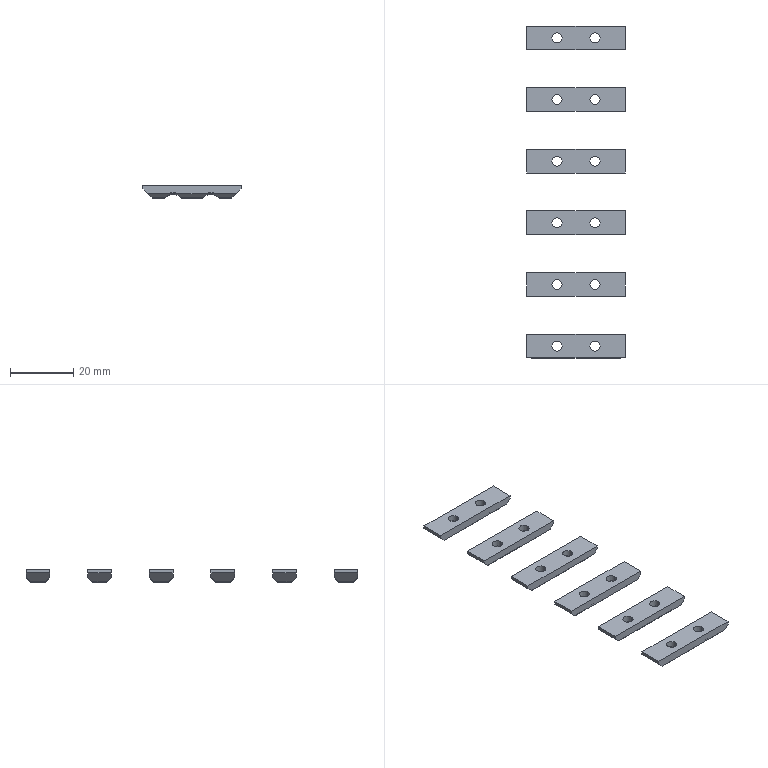NC program | NX | posted with a generic post | part box 31 x 105 x 4 mm
Lines 5449 to 7045 of 12738:
(PLANAR_MILL , TOOL : D0.3)
N10860 T17 M6
N10862 G54
N10864 G17 G0 G90 X-45.35 Y-12.5 S9500 M3
N10866 G43 Z30. H17
N10868 Z0.97
N10870 G94 G1 Z-0.03 F750.
N10872 X-46.5
N10874 X-51.
N10876 X-52.15
N10878 Z0.97
N10880 G0 Z30.
N10882 X-45.35 Y-12.
N10884 Z0.97
N10886 G1 Z-0.03
N10888 X-46.5
N10890 X-51.
N10892 X-52.15
N10894 Z0.97
N10896 G0 Z30.
N10898 X-45.35 Y-11.5
N10900 Z0.97
N10902 G1 Z-0.03
N10904 X-46.5
N10906 X-51.
N10908 X-52.15
N10910 Z0.97
N10912 G0 Z30.
N10914 X-45.35 Y-11.
N10916 Z0.97
N10918 G1 Z-0.03
N10920 X-46.5
N10922 X-51.
N10924 X-52.15
N10926 Z0.97
N10928 G0 Z30.
N10930 X-45.35 Y-10.5
N10932 Z0.97
N10934 G1 Z-0.03
N10936 X-46.5
N10938 X-51.
N10940 X-52.15
N10942 Z0.97
N10944 G0 Z30.
N10946 X-45.35 Y-10.
N10948 Z0.97
N10950 G1 Z-0.03
N10952 X-46.5
N10954 X-51.
N10956 X-52.15
N10958 Z0.97
N10960 G0 Z30.
N10962 X-45.35 Y-9.5
N10964 Z0.97
N10966 G1 Z-0.03
N10968 X-46.5
N10970 X-51.
N10972 X-52.15
N10974 Z0.97
N10976 G0 Z30.
N10978 X-45.35 Y-9.
N10980 Z0.97
N10982 G1 Z-0.03
N10984 X-46.5
N10986 X-51.
N10988 X-52.15
N10990 Z0.97
N10992 G0 Z30.
N10994 X-45.35 Y-3.
N10996 Z0.97
N10998 G1 Z-0.03
N11000 X-46.5
N11002 X-51.
N11004 X-52.15
N11006 Z0.97
N11008 G0 Z30.
N11010 X-45.35 Y-2.5
N11012 Z0.97
N11014 G1 Z-0.03
N11016 X-46.5
N11018 X-51.
N11020 X-52.15
N11022 Z0.97
N11024 G0 Z30.
N11026 X-45.35 Y-2.
N11028 Z0.97
N11030 G1 Z-0.03
N11032 X-46.5
N11034 X-51.
N11036 X-52.15
N11038 Z0.97
N11040 G0 Z30.
N11042 X-45.35 Y-1.5
N11044 Z0.97
N11046 G1 Z-0.03
N11048 X-46.5
N11050 X-51.
N11052 X-52.15
N11054 Z0.97
N11056 G0 Z30.
N11058 X-45.35 Y-1.
N11060 Z0.97
N11062 G1 Z-0.03
N11064 X-46.5
N11066 X-51.
N11068 X-52.15
N11070 Z0.97
N11072 G0 Z30.
N11074 X-45.35 Y-0.5
N11076 Z0.97
N11078 G1 Z-0.03
N11080 X-46.5
N11082 X-51.
N11084 X-52.15
N11086 Z0.97
N11088 G0 Z30.
N11090 X-45.35 Y0.
N11092 Z0.97
N11094 G1 Z-0.03
N11096 X-46.5
N11098 X-51.
N11100 X-52.15
N11102 Z0.97
N11104 G0 Z30.
N11106 X-45.35 Y0.5
N11108 Z0.97
N11110 G1 Z-0.03
N11112 X-46.5
N11114 X-51.
N11116 X-52.15
N11118 Z0.97
N11120 G0 Z30.
N11122 X-45.35 Y1.
N11124 Z0.97
N11126 G1 Z-0.03
N11128 X-46.5
N11130 X-51.
N11132 X-52.15
N11134 Z0.97
N11136 G0 Z30.
N11138 X-45.35 Y1.5
N11140 Z0.97
N11142 G1 Z-0.03
N11144 X-46.5
N11146 X-51.
N11148 X-52.15
N11150 Z0.97
N11152 G0 Z30.
N11154 X-45.35 Y2.
N11156 Z0.97
N11158 G1 Z-0.03
N11160 X-46.5
N11162 X-51.
N11164 X-52.15
N11166 Z0.97
N11168 G0 Z30.
N11170 X-45.35 Y2.5
N11172 Z0.97
N11174 G1 Z-0.03
N11176 X-46.5
N11178 X-51.
N11180 X-52.15
N11182 Z0.97
N11184 G0 Z30.
N11186 X-45.35 Y3.
N11188 Z0.97
N11190 G1 Z-0.03
N11192 X-46.5
N11194 X-51.
N11196 X-52.15
N11198 Z0.97
N11200 G0 Z30.
N11202 X-45.35 Y9.
N11204 Z0.97
N11206 G1 Z-0.03
N11208 X-46.5
N11210 X-51.
N11212 X-52.15
N11214 Z0.97
N11216 G0 Z30.
N11218 X-45.35 Y9.5
N11220 Z0.97
N11222 G1 Z-0.03
N11224 X-46.5
N11226 X-51.
N11228 X-52.15
N11230 Z0.97
N11232 G0 Z30.
N11234 X-45.35 Y10.
N11236 Z0.97
N11238 G1 Z-0.03
N11240 X-46.5
N11242 X-51.
N11244 X-52.15
N11246 Z0.97
N11248 G0 Z30.
N11250 X-45.35 Y10.5
N11252 Z0.97
N11254 G1 Z-0.03
N11256 X-46.5
N11258 X-51.
N11260 X-52.15
N11262 Z0.97
N11264 G0 Z30.
N11266 X-45.35 Y11.
N11268 Z0.97
N11270 G1 Z-0.03
N11272 X-46.5
N11274 X-51.
N11276 X-52.15
N11278 Z0.97
N11280 G0 Z30.
N11282 X-45.35 Y11.5
N11284 Z0.97
N11286 G1 Z-0.03
N11288 X-46.5
N11290 X-51.
N11292 X-52.15
N11294 Z0.97
N11296 G0 Z30.
N11298 X-45.2 Y12.
N11300 Z0.97
N11302 G1 Z-0.03
N11304 X-46.5
N11306 X-51.
N11308 X-52.3
N11310 Z0.97
N11312 G0 Z30.
N11314 X-45.2 Y12.5
N11316 Z0.97
N11318 G1 Z-0.03
N11320 X-46.35
N11322 X-51.15
N11324 X-52.3
N11326 Z0.97
N11328 G0 Z30.
N11330 X-45.2
N11332 Z0.94
N11334 G1 Z-0.06
N11336 X-46.35
N11338 X-51.15
N11340 X-52.3
N11342 Z0.94
N11344 G0 Z30.
N11346 X-45.2 Y12.
N11348 Z0.94
N11350 G1 Z-0.06
N11352 X-46.5
N11354 X-51.
N11356 X-52.3
N11358 Z0.94
N11360 G0 Z30.
N11362 X-45.35 Y11.5
N11364 Z0.94
N11366 G1 Z-0.06
N11368 X-46.5
N11370 X-51.
N11372 X-52.15
N11374 Z0.94
N11376 G0 Z30.
N11378 X-45.35 Y11.
N11380 Z0.94
N11382 G1 Z-0.06
N11384 X-46.5
N11386 X-51.
N11388 X-52.15
N11390 Z0.94
N11392 G0 Z30.
N11394 X-45.35 Y10.5
N11396 Z0.94
N11398 G1 Z-0.06
N11400 X-46.5
N11402 X-51.
N11404 X-52.15
N11406 Z0.94
N11408 G0 Z30.
N11410 X-45.35 Y10.
N11412 Z0.94
N11414 G1 Z-0.06
N11416 X-46.5
N11418 X-51.
N11420 X-52.15
N11422 Z0.94
N11424 G0 Z30.
N11426 X-45.35 Y9.5
N11428 Z0.94
N11430 G1 Z-0.06
N11432 X-46.5
N11434 X-51.
N11436 X-52.15
N11438 Z0.94
N11440 G0 Z30.
N11442 X-45.35 Y9.
N11444 Z0.94
N11446 G1 Z-0.06
N11448 X-46.5
N11450 X-51.
N11452 X-52.15
N11454 Z0.94
N11456 G0 Z30.
N11458 X-45.35 Y3.
N11460 Z0.94
N11462 G1 Z-0.06
N11464 X-46.5
N11466 X-51.
N11468 X-52.15
N11470 Z0.94
N11472 G0 Z30.
N11474 X-45.35 Y2.5
N11476 Z0.94
N11478 G1 Z-0.06
N11480 X-46.5
N11482 X-51.
N11484 X-52.15
N11486 Z0.94
N11488 G0 Z30.
N11490 X-45.35 Y2.
N11492 Z0.94
N11494 G1 Z-0.06
N11496 X-46.5
N11498 X-51.
N11500 X-52.15
N11502 Z0.94
N11504 G0 Z30.
N11506 X-45.35 Y1.5
N11508 Z0.94
N11510 G1 Z-0.06
N11512 X-46.5
N11514 X-51.
N11516 X-52.15
N11518 Z0.94
N11520 G0 Z30.
N11522 X-45.35 Y1.
N11524 Z0.94
N11526 G1 Z-0.06
N11528 X-46.5
N11530 X-51.
N11532 X-52.15
N11534 Z0.94
N11536 G0 Z30.
N11538 X-45.35 Y0.5
N11540 Z0.94
N11542 G1 Z-0.06
N11544 X-46.5
N11546 X-51.
N11548 X-52.15
N11550 Z0.94
N11552 G0 Z30.
N11554 X-45.35 Y0.
N11556 Z0.94
N11558 G1 Z-0.06
N11560 X-46.5
N11562 X-51.
N11564 X-52.15
N11566 Z0.94
N11568 G0 Z30.
N11570 X-45.35 Y-0.5
N11572 Z0.94
N11574 G1 Z-0.06
N11576 X-46.5
N11578 X-51.
N11580 X-52.15
N11582 Z0.94
N11584 G0 Z30.
N11586 X-45.35 Y-1.
N11588 Z0.94
N11590 G1 Z-0.06
N11592 X-46.5
N11594 X-51.
N11596 X-52.15
N11598 Z0.94
N11600 G0 Z30.
N11602 X-45.35 Y-1.5
N11604 Z0.94
N11606 G1 Z-0.06
N11608 X-46.5
N11610 X-51.
N11612 X-52.15
N11614 Z0.94
N11616 G0 Z30.
N11618 X-45.35 Y-2.
N11620 Z0.94
N11622 G1 Z-0.06
N11624 X-46.5
N11626 X-51.
N11628 X-52.15
N11630 Z0.94
N11632 G0 Z30.
N11634 X-45.35 Y-2.5
N11636 Z0.94
N11638 G1 Z-0.06
N11640 X-46.5
N11642 X-51.
N11644 X-52.15
N11646 Z0.94
N11648 G0 Z30.
N11650 X-45.35 Y-3.
N11652 Z0.94
N11654 G1 Z-0.06
N11656 X-46.5
N11658 X-51.
N11660 X-52.15
N11662 Z0.94
N11664 G0 Z30.
N11666 X-45.35 Y-9.
N11668 Z0.94
N11670 G1 Z-0.06
N11672 X-46.5
N11674 X-51.
N11676 X-52.15
N11678 Z0.94
N11680 G0 Z30.
N11682 X-45.35 Y-9.5
N11684 Z0.94
N11686 G1 Z-0.06
N11688 X-46.5
N11690 X-51.
N11692 X-52.15
N11694 Z0.94
N11696 G0 Z30.
N11698 X-45.35 Y-10.
N11700 Z0.94
N11702 G1 Z-0.06
N11704 X-46.5
N11706 X-51.
N11708 X-52.15
N11710 Z0.94
N11712 G0 Z30.
N11714 X-45.35 Y-10.5
N11716 Z0.94
N11718 G1 Z-0.06
N11720 X-46.5
N11722 X-51.
N11724 X-52.15
N11726 Z0.94
N11728 G0 Z30.
N11730 X-45.35 Y-11.
N11732 Z0.94
N11734 G1 Z-0.06
N11736 X-46.5
N11738 X-51.
N11740 X-52.15
N11742 Z0.94
N11744 G0 Z30.
N11746 X-45.35 Y-11.5
N11748 Z0.94
N11750 G1 Z-0.06
N11752 X-46.5
N11754 X-51.
N11756 X-52.15
N11758 Z0.94
N11760 G0 Z30.
N11762 X-45.35 Y-12.
N11764 Z0.94
N11766 G1 Z-0.06
N11768 X-46.5
N11770 X-51.
N11772 X-52.15
N11774 Z0.94
N11776 G0 Z30.
N11778 X-45.35 Y-12.5
N11780 Z0.94
N11782 G1 Z-0.06
N11784 X-46.5
N11786 X-51.
N11788 X-52.15
N11790 Z0.94
N11792 G0 Z30.
N11794 X-45.35
N11796 Z0.91
N11798 G1 Z-0.09
N11800 X-46.5
N11802 X-51.
N11804 X-52.15
N11806 Z0.91
N11808 G0 Z30.
N11810 X-45.35 Y-12.
N11812 Z0.91
N11814 G1 Z-0.09
N11816 X-46.5
N11818 X-51.
N11820 X-52.15
N11822 Z0.91
N11824 G0 Z30.
N11826 X-45.35 Y-11.5
N11828 Z0.91
N11830 G1 Z-0.09
N11832 X-46.5
N11834 X-51.
N11836 X-52.15
N11838 Z0.91
N11840 G0 Z30.
N11842 X-45.35 Y-11.
N11844 Z0.91
N11846 G1 Z-0.09
N11848 X-46.5
N11850 X-51.
N11852 X-52.15
N11854 Z0.91
N11856 G0 Z30.
N11858 X-45.35 Y-10.5
N11860 Z0.91
N11862 G1 Z-0.09
N11864 X-46.5
N11866 X-51.
N11868 X-52.15
N11870 Z0.91
N11872 G0 Z30.
N11874 X-45.35 Y-10.
N11876 Z0.91
N11878 G1 Z-0.09
N11880 X-46.5
N11882 X-51.
N11884 X-52.15
N11886 Z0.91
N11888 G0 Z30.
N11890 X-45.35 Y-9.5
N11892 Z0.91
N11894 G1 Z-0.09
N11896 X-46.5
N11898 X-51.
N11900 X-52.15
N11902 Z0.91
N11904 G0 Z30.
N11906 X-45.35 Y-9.
N11908 Z0.91
N11910 G1 Z-0.09
N11912 X-46.5
N11914 X-51.
N11916 X-52.15
N11918 Z0.91
N11920 G0 Z30.
N11922 X-45.35 Y-3.
N11924 Z0.91
N11926 G1 Z-0.09
N11928 X-46.5
N11930 X-51.
N11932 X-52.15
N11934 Z0.91
N11936 G0 Z30.
N11938 X-45.35 Y-2.5
N11940 Z0.91
N11942 G1 Z-0.09
N11944 X-46.5
N11946 X-51.
N11948 X-52.15
N11950 Z0.91
N11952 G0 Z30.
N11954 X-45.35 Y-2.
N11956 Z0.91
N11958 G1 Z-0.09
N11960 X-46.5
N11962 X-51.
N11964 X-52.15
N11966 Z0.91
N11968 G0 Z30.
N11970 X-45.35 Y-1.5
N11972 Z0.91
N11974 G1 Z-0.09
N11976 X-46.5
N11978 X-51.
N11980 X-52.15
N11982 Z0.91
N11984 G0 Z30.
N11986 X-45.35 Y-1.
N11988 Z0.91
N11990 G1 Z-0.09
N11992 X-46.5
N11994 X-51.
N11996 X-52.15
N11998 Z0.91
N12000 G0 Z30.
N12002 X-45.35 Y-0.5
N12004 Z0.91
N12006 G1 Z-0.09
N12008 X-46.5
N12010 X-51.
N12012 X-52.15
N12014 Z0.91
N12016 G0 Z30.
N12018 X-45.35 Y0.
N12020 Z0.91
N12022 G1 Z-0.09
N12024 X-46.5
N12026 X-51.
N12028 X-52.15
N12030 Z0.91
N12032 G0 Z30.
N12034 X-45.35 Y0.5
N12036 Z0.91
N12038 G1 Z-0.09
N12040 X-46.5
N12042 X-51.
N12044 X-52.15
N12046 Z0.91
N12048 G0 Z30.
N12050 X-45.35 Y1.
N12052 Z0.91
N12054 G1 Z-0.09
N12056 X-46.5
N12058 X-51.
N12060 X-52.15
N12062 Z0.91
N12064 G0 Z30.
N12066 X-45.35 Y1.5
N12068 Z0.91
N12070 G1 Z-0.09
N12072 X-46.5
N12074 X-51.
N12076 X-52.15
N12078 Z0.91
N12080 G0 Z30.
N12082 X-45.35 Y2.
N12084 Z0.91
N12086 G1 Z-0.09
N12088 X-46.5
N12090 X-51.
N12092 X-52.15
N12094 Z0.91
N12096 G0 Z30.
N12098 X-45.35 Y2.5
N12100 Z0.91
N12102 G1 Z-0.09
N12104 X-46.5
N12106 X-51.
N12108 X-52.15
N12110 Z0.91
N12112 G0 Z30.
N12114 X-45.35 Y3.
N12116 Z0.91
N12118 G1 Z-0.09
N12120 X-46.5
N12122 X-51.
N12124 X-52.15
N12126 Z0.91
N12128 G0 Z30.
N12130 X-45.35 Y9.
N12132 Z0.91
N12134 G1 Z-0.09
N12136 X-46.5
N12138 X-51.
N12140 X-52.15
N12142 Z0.91
N12144 G0 Z30.
N12146 X-45.35 Y9.5
N12148 Z0.91
N12150 G1 Z-0.09
N12152 X-46.5
N12154 X-51.
N12156 X-52.15
N12158 Z0.91
N12160 G0 Z30.
N12162 X-45.35 Y10.
N12164 Z0.91
N12166 G1 Z-0.09
N12168 X-46.5
N12170 X-51.
N12172 X-52.15
N12174 Z0.91
N12176 G0 Z30.
N12178 X-45.35 Y10.5
N12180 Z0.91
N12182 G1 Z-0.09
N12184 X-46.5
N12186 X-51.
N12188 X-52.15
N12190 Z0.91
N12192 G0 Z30.
N12194 X-45.35 Y11.
N12196 Z0.91
N12198 G1 Z-0.09
N12200 X-46.5
N12202 X-51.
N12204 X-52.15
N12206 Z0.91
N12208 G0 Z30.
N12210 X-45.35 Y11.5
N12212 Z0.91
N12214 G1 Z-0.09
N12216 X-46.5
N12218 X-51.
N12220 X-52.15
N12222 Z0.91
N12224 G0 Z30.
N12226 X-45.2 Y12.
N12228 Z0.91
N12230 G1 Z-0.09
N12232 X-46.5
N12234 X-51.
N12236 X-52.3
N12238 Z0.91
N12240 G0 Z30.
N12242 X-45.2 Y12.5
N12244 Z0.91
N12246 G1 Z-0.09
N12248 X-46.35
N12250 X-51.15
N12252 X-52.3
N12254 Z0.91
N12256 G0 Z30.
N12258 X-45.2
N12260 Z0.88
N12262 G1 Z-0.12
N12264 X-46.35
N12266 X-51.15
N12268 X-52.3
N12270 Z0.88
N12272 G0 Z30.
N12274 X-45.2 Y12.
N12276 Z0.88
N12278 G1 Z-0.12
N12280 X-46.5
N12282 X-51.
N12284 X-52.3
N12286 Z0.88
N12288 G0 Z30.
N12290 X-45.35 Y11.5
N12292 Z0.88
N12294 G1 Z-0.12
N12296 X-46.5
N12298 X-51.
N12300 X-52.15
N12302 Z0.88
N12304 G0 Z30.
N12306 X-45.35 Y11.
N12308 Z0.88
N12310 G1 Z-0.12
N12312 X-46.5
N12314 X-51.
N12316 X-52.15
N12318 Z0.88
N12320 G0 Z30.
N12322 X-45.35 Y10.5
N12324 Z0.88
N12326 G1 Z-0.12
N12328 X-46.5
N12330 X-51.
N12332 X-52.15
N12334 Z0.88
N12336 G0 Z30.
N12338 X-45.35 Y10.
N12340 Z0.88
N12342 G1 Z-0.12
N12344 X-46.5
N12346 X-51.
N12348 X-52.15
N12350 Z0.88
N12352 G0 Z30.
N12354 X-45.35 Y9.5
N12356 Z0.88
N12358 G1 Z-0.12
N12360 X-46.5
N12362 X-51.
N12364 X-52.15
N12366 Z0.88
N12368 G0 Z30.
N12370 X-45.35 Y9.
N12372 Z0.88
N12374 G1 Z-0.12
N12376 X-46.5
N12378 X-51.
N12380 X-52.15
N12382 Z0.88
N12384 G0 Z30.
N12386 X-45.35 Y3.
N12388 Z0.88
N12390 G1 Z-0.12
N12392 X-46.5
N12394 X-51.
N12396 X-52.15
N12398 Z0.88
N12400 G0 Z30.
N12402 X-45.35 Y2.5
N12404 Z0.88
N12406 G1 Z-0.12
N12408 X-46.5
N12410 X-51.
N12412 X-52.15
N12414 Z0.88
N12416 G0 Z30.
N12418 X-45.35 Y2.
N12420 Z0.88
N12422 G1 Z-0.12
N12424 X-46.5
N12426 X-51.
N12428 X-52.15
N12430 Z0.88
N12432 G0 Z30.
N12434 X-45.35 Y1.5
N12436 Z0.88
N12438 G1 Z-0.12
N12440 X-46.5
N12442 X-51.
N12444 X-52.15
N12446 Z0.88
N12448 G0 Z30.
N12450 X-45.35 Y1.
N12452 Z0.88
N12454 G1 Z-0.12
N12456 X-46.5
N12458 X-51.
N12460 X-52.15
N12462 Z0.88
N12464 G0 Z30.
N12466 X-45.35 Y0.5
N12468 Z0.88
N12470 G1 Z-0.12
N12472 X-46.5
N12474 X-51.
N12476 X-52.15
N12478 Z0.88
N12480 G0 Z30.
N12482 X-45.35 Y0.
N12484 Z0.88
N12486 G1 Z-0.12
N12488 X-46.5
N12490 X-51.
N12492 X-52.15
N12494 Z0.88
N12496 G0 Z30.
N12498 X-45.35 Y-0.5
N12500 Z0.88
N12502 G1 Z-0.12
N12504 X-46.5
N12506 X-51.
N12508 X-52.15
N12510 Z0.88
N12512 G0 Z30.
N12514 X-45.35 Y-1.
N12516 Z0.88
N12518 G1 Z-0.12
N12520 X-46.5
N12522 X-51.
N12524 X-52.15
N12526 Z0.88
N12528 G0 Z30.
N12530 X-45.35 Y-1.5
N12532 Z0.88
N12534 G1 Z-0.12
N12536 X-46.5
N12538 X-51.
N12540 X-52.15
N12542 Z0.88
N12544 G0 Z30.
N12546 X-45.35 Y-2.
N12548 Z0.88
N12550 G1 Z-0.12
N12552 X-46.5
N12554 X-51.
N12556 X-52.15
N12558 Z0.88
N12560 G0 Z30.
N12562 X-45.35 Y-2.5
N12564 Z0.88
N12566 G1 Z-0.12
N12568 X-46.5
N12570 X-51.
N12572 X-52.15
N12574 Z0.88
N12576 G0 Z30.
N12578 X-45.35 Y-3.
N12580 Z0.88
N12582 G1 Z-0.12
N12584 X-46.5
N12586 X-51.
N12588 X-52.15
N12590 Z0.88
N12592 G0 Z30.
N12594 X-45.35 Y-9.
N12596 Z0.88
N12598 G1 Z-0.12
N12600 X-46.5
N12602 X-51.
N12604 X-52.15
N12606 Z0.88
N12608 G0 Z30.
N12610 X-45.35 Y-9.5
N12612 Z0.88
N12614 G1 Z-0.12
N12616 X-46.5
N12618 X-51.
N12620 X-52.15
N12622 Z0.88
N12624 G0 Z30.
N12626 X-45.35 Y-10.
N12628 Z0.88
N12630 G1 Z-0.12
N12632 X-46.5
N12634 X-51.
N12636 X-52.15
N12638 Z0.88
N12640 G0 Z30.
N12642 X-45.35 Y-10.5
N12644 Z0.88
N12646 G1 Z-0.12
N12648 X-46.5
N12650 X-51.
N12652 X-52.15
N12654 Z0.88
N12656 G0 Z30.
N12658 X-45.35 Y-11.
N12660 Z0.88
N12662 G1 Z-0.12
N12664 X-46.5
N12666 X-51.
N12668 X-52.15
N12670 Z0.88
N12672 G0 Z30.
N12674 X-45.35 Y-11.5
N12676 Z0.88
N12678 G1 Z-0.12
N12680 X-46.5
N12682 X-51.
N12684 X-52.15
N12686 Z0.88
N12688 G0 Z30.
N12690 X-45.35 Y-12.
N12692 Z0.88
N12694 G1 Z-0.12
N12696 X-46.5
N12698 X-51.
N12700 X-52.15
N12702 Z0.88
N12704 G0 Z30.
N12706 X-45.35 Y-12.5
N12708 Z0.88
N12710 G1 Z-0.12
N12712 X-46.5
N12714 X-51.
N12716 X-52.15
N12718 Z0.88
N12720 G0 Z30.
N12722 X-45.35
N12724 Z0.85
N12726 G1 Z-0.15
N12728 X-46.5
N12730 X-51.
N12732 X-52.15
N12734 Z0.85
N12736 G0 Z30.
N12738 X-45.35 Y-12.
N12740 Z0.85
N12742 G1 Z-0.15
N12744 X-46.5
N12746 X-51.
N12748 X-52.15
N12750 Z0.85
N12752 G0 Z30.
N12754 X-45.35 Y-11.5
N12756 Z0.85
N12758 G1 Z-0.15
N12760 X-46.5
N12762 X-51.
N12764 X-52.15
N12766 Z0.85
N12768 G0 Z30.
N12770 X-45.35 Y-11.
N12772 Z0.85
N12774 G1 Z-0.15
N12776 X-46.5
N12778 X-51.
N12780 X-52.15
N12782 Z0.85
N12784 G0 Z30.
N12786 X-45.35 Y-10.5
N12788 Z0.85
N12790 G1 Z-0.15
N12792 X-46.5
N12794 X-51.
N12796 X-52.15
N12798 Z0.85
N12800 G0 Z30.
N12802 X-45.35 Y-10.
N12804 Z0.85
N12806 G1 Z-0.15
N12808 X-46.5
N12810 X-51.
N12812 X-52.15
N12814 Z0.85
N12816 G0 Z30.
N12818 X-45.35 Y-9.5
N12820 Z0.85
N12822 G1 Z-0.15
N12824 X-46.5
N12826 X-51.
N12828 X-52.15
N12830 Z0.85
N12832 G0 Z30.
N12834 X-45.35 Y-9.
N12836 Z0.85
N12838 G1 Z-0.15
N12840 X-46.5
N12842 X-51.
N12844 X-52.15
N12846 Z0.85
N12848 G0 Z30.
N12850 X-45.35 Y-3.
N12852 Z0.85
N12854 G1 Z-0.15
N12856 X-46.5
N12858 X-51.
N12860 X-52.15
N12862 Z0.85
N12864 G0 Z30.
N12866 X-45.35 Y-2.5
N12868 Z0.85
N12870 G1 Z-0.15
N12872 X-46.5
N12874 X-51.
N12876 X-52.15
N12878 Z0.85
N12880 G0 Z30.
N12882 X-45.35 Y-2.
N12884 Z0.85
N12886 G1 Z-0.15
N12888 X-46.5
N12890 X-51.
N12892 X-52.15
N12894 Z0.85
N12896 G0 Z30.
N12898 X-45.35 Y-1.5
N12900 Z0.85
N12902 G1 Z-0.15
N12904 X-46.5
N12906 X-51.
N12908 X-52.15
N12910 Z0.85
N12912 G0 Z30.
N12914 X-45.35 Y-1.
N12916 Z0.85
N12918 G1 Z-0.15
N12920 X-46.5
N12922 X-51.
N12924 X-52.15
N12926 Z0.85
N12928 G0 Z30.
N12930 X-45.35 Y-0.5
N12932 Z0.85
N12934 G1 Z-0.15
N12936 X-46.5
N12938 X-51.
N12940 X-52.15
N12942 Z0.85
N12944 G0 Z30.
N12946 X-45.35 Y0.
N12948 Z0.85
N12950 G1 Z-0.15
N12952 X-46.5
N12954 X-51.
N12956 X-52.15
N12958 Z0.85
N12960 G0 Z30.
N12962 X-45.35 Y0.5
N12964 Z0.85
N12966 G1 Z-0.15
N12968 X-46.5
N12970 X-51.
N12972 X-52.15
N12974 Z0.85
N12976 G0 Z30.
N12978 X-45.35 Y1.
N12980 Z0.85
N12982 G1 Z-0.15
N12984 X-46.5
N12986 X-51.
N12988 X-52.15
N12990 Z0.85
N12992 G0 Z30.
N12994 X-45.35 Y1.5
N12996 Z0.85
N12998 G1 Z-0.15
N13000 X-46.5
N13002 X-51.
N13004 X-52.15
N13006 Z0.85
N13008 G0 Z30.
N13010 X-45.35 Y2.
N13012 Z0.85
N13014 G1 Z-0.15
N13016 X-46.5
N13018 X-51.
N13020 X-52.15
N13022 Z0.85
N13024 G0 Z30.
N13026 X-45.35 Y2.5
N13028 Z0.85
N13030 G1 Z-0.15
N13032 X-46.5
N13034 X-51.
N13036 X-52.15
N13038 Z0.85
N13040 G0 Z30.
N13042 X-45.35 Y3.
N13044 Z0.85
N13046 G1 Z-0.15
N13048 X-46.5
N13050 X-51.
N13052 X-52.15
N13054 Z0.85
N13056 G0 Z30.
N13058 X-45.35 Y9.
N13060 Z0.85
N13062 G1 Z-0.15
N13064 X-46.5
N13066 X-51.
N13068 X-52.15
N13070 Z0.85
N13072 G0 Z30.
N13074 X-45.35 Y9.5
N13076 Z0.85
N13078 G1 Z-0.15
N13080 X-46.5
N13082 X-51.
N13084 X-52.15
N13086 Z0.85
N13088 G0 Z30.
N13090 X-45.35 Y10.
N13092 Z0.85
N13094 G1 Z-0.15
N13096 X-46.5
N13098 X-51.
N13100 X-52.15
N13102 Z0.85
N13104 G0 Z30.
N13106 X-45.35 Y10.5
N13108 Z0.85
N13110 G1 Z-0.15
N13112 X-46.5
N13114 X-51.
N13116 X-52.15
N13118 Z0.85
N13120 G0 Z30.
N13122 X-45.35 Y11.
N13124 Z0.85
N13126 G1 Z-0.15
N13128 X-46.5
N13130 X-51.
N13132 X-52.15
N13134 Z0.85
N13136 G0 Z30.
N13138 X-45.35 Y11.5
N13140 Z0.85
N13142 G1 Z-0.15
N13144 X-46.5
N13146 X-51.
N13148 X-52.15
N13150 Z0.85
N13152 G0 Z30.
N13154 X-45.2 Y12.
N13156 Z0.85
N13158 G1 Z-0.15
N13160 X-46.5
N13162 X-51.
N13164 X-52.3
N13166 Z0.85
N13168 G0 Z30.
N13170 X-45.2 Y12.5
N13172 Z0.85
N13174 G1 Z-0.15
N13176 X-46.35
N13178 X-51.15
N13180 X-52.3
N13182 Z0.85
N13184 G0 Z30.
(PLANAR_MILL_COPY , TOOL : D0.3)
N13186 X-25.85 Y-12.5
N13188 Z0.97
N13190 G1 Z-0.03
N13192 X-27.
N13194 X-31.5
N13196 X-32.65
N13198 Z0.97
N13200 G0 Z30.
N13202 X-25.85 Y-12.
N13204 Z0.97
N13206 G1 Z-0.03
N13208 X-27.
N13210 X-31.5
N13212 X-32.65
N13214 Z0.97
N13216 G0 Z30.
N13218 X-25.85 Y-11.5
N13220 Z0.97
N13222 G1 Z-0.03
N13224 X-27.
N13226 X-31.5
N13228 X-32.65
N13230 Z0.97
N13232 G0 Z30.
N13234 X-25.85 Y-11.
N13236 Z0.97
N13238 G1 Z-0.03
N13240 X-27.
N13242 X-31.5
N13244 X-32.65
N13246 Z0.97
N13248 G0 Z30.
N13250 X-25.85 Y-10.5
N13252 Z0.97
N13254 G1 Z-0.03
N13256 X-27.
N13258 X-31.5
N13260 X-32.65
N13262 Z0.97
N13264 G0 Z30.
N13266 X-25.85 Y-10.
N13268 Z0.97
N13270 G1 Z-0.03
N13272 X-27.
N13274 X-31.5
N13276 X-32.65
N13278 Z0.97
N13280 G0 Z30.
N13282 X-25.85 Y-9.5
N13284 Z0.97
N13286 G1 Z-0.03
N13288 X-27.
N13290 X-31.5
N13292 X-32.65
N13294 Z0.97
N13296 G0 Z30.
N13298 X-25.85 Y-9.
N13300 Z0.97
N13302 G1 Z-0.03
N13304 X-27.
N13306 X-31.5
N13308 X-32.65
N13310 Z0.97
N13312 G0 Z30.
N13314 X-25.85 Y-3.
N13316 Z0.97
N13318 G1 Z-0.03
N13320 X-27.
N13322 X-31.5
N13324 X-32.65
N13326 Z0.97
N13328 G0 Z30.
N13330 X-25.85 Y-2.5
N13332 Z0.97
N13334 G1 Z-0.03
N13336 X-27.
N13338 X-31.5
N13340 X-32.65
N13342 Z0.97
N13344 G0 Z30.
N13346 X-25.85 Y-2.
N13348 Z0.97
N13350 G1 Z-0.03
N13352 X-27.
N13354 X-31.5
N13356 X-32.65
N13358 Z0.97
N13360 G0 Z30.
N13362 X-25.85 Y-1.5
N13364 Z0.97
N13366 G1 Z-0.03
N13368 X-27.
N13370 X-31.5
N13372 X-32.65
N13374 Z0.97
N13376 G0 Z30.
N13378 X-25.85 Y-1.
N13380 Z0.97
N13382 G1 Z-0.03
N13384 X-27.
N13386 X-31.5
N13388 X-32.65
N13390 Z0.97
N13392 G0 Z30.
N13394 X-25.85 Y-0.5
N13396 Z0.97
N13398 G1 Z-0.03
N13400 X-27.
N13402 X-31.5
N13404 X-32.65
N13406 Z0.97
N13408 G0 Z30.
N13410 X-25.85 Y0.
N13412 Z0.97
N13414 G1 Z-0.03
N13416 X-27.
N13418 X-31.5
N13420 X-32.65
N13422 Z0.97
N13424 G0 Z30.
N13426 X-25.85 Y0.5
N13428 Z0.97
N13430 G1 Z-0.03
N13432 X-27.
N13434 X-31.5
N13436 X-32.65
N13438 Z0.97
N13440 G0 Z30.
N13442 X-25.85 Y1.
N13444 Z0.97
N13446 G1 Z-0.03
N13448 X-27.
N13450 X-31.5
N13452 X-32.65
N13454 Z0.97
N13456 G0 Z30.
N13458 X-25.85 Y1.5
N13460 Z0.97
N13462 G1 Z-0.03
N13464 X-27.
N13466 X-31.5
N13468 X-32.65
N13470 Z0.97
N13472 G0 Z30.
N13474 X-25.85 Y2.
N13476 Z0.97
N13478 G1 Z-0.03
N13480 X-27.
N13482 X-31.5
N13484 X-32.65
N13486 Z0.97
N13488 G0 Z30.
N13490 X-25.85 Y2.5
N13492 Z0.97
N13494 G1 Z-0.03
N13496 X-27.
N13498 X-31.5
N13500 X-32.65
N13502 Z0.97
N13504 G0 Z30.
N13506 X-25.85 Y3.
N13508 Z0.97
N13510 G1 Z-0.03
N13512 X-27.
N13514 X-31.5
N13516 X-32.65
N13518 Z0.97
N13520 G0 Z30.
N13522 X-25.85 Y9.
N13524 Z0.97
N13526 G1 Z-0.03
N13528 X-27.
N13530 X-31.5
N13532 X-32.65
N13534 Z0.97
N13536 G0 Z30.
N13538 X-25.85 Y9.5
N13540 Z0.97
N13542 G1 Z-0.03
N13544 X-27.
N13546 X-31.5
N13548 X-32.65
N13550 Z0.97
N13552 G0 Z30.
N13554 X-25.85 Y10.
N13556 Z0.97
N13558 G1 Z-0.03
N13560 X-27.
N13562 X-31.5
N13564 X-32.65
N13566 Z0.97
N13568 G0 Z30.
N13570 X-25.85 Y10.5
N13572 Z0.97
N13574 G1 Z-0.03
N13576 X-27.
N13578 X-31.5
N13580 X-32.65
N13582 Z0.97
N13584 G0 Z30.
N13586 X-25.85 Y11.
N13588 Z0.97
N13590 G1 Z-0.03
N13592 X-27.
N13594 X-31.5
N13596 X-32.65
N13598 Z0.97
N13600 G0 Z30.
N13602 X-25.85 Y11.5
N13604 Z0.97
N13606 G1 Z-0.03
N13608 X-27.
N13610 X-31.5
N13612 X-32.65
N13614 Z0.97
N13616 G0 Z30.
N13618 X-25.7 Y12.
N13620 Z0.97
N13622 G1 Z-0.03
N13624 X-27.
N13626 X-31.5
N13628 X-32.8
N13630 Z0.97
N13632 G0 Z30.
N13634 X-25.7 Y12.5
N13636 Z0.97
N13638 G1 Z-0.03
N13640 X-26.85
N13642 X-31.65
N13644 X-32.8
N13646 Z0.97
N13648 G0 Z30.
N13650 X-25.7
N13652 Z0.94
N13654 G1 Z-0.06
N13656 X-26.85
N13658 X-31.65
N13660 X-32.8
N13662 Z0.94
N13664 G0 Z30.
N13666 X-25.7 Y12.
N13668 Z0.94
N13670 G1 Z-0.06
N13672 X-27.
N13674 X-31.5
N13676 X-32.8
N13678 Z0.94
N13680 G0 Z30.
N13682 X-25.85 Y11.5
N13684 Z0.94
N13686 G1 Z-0.06
N13688 X-27.
N13690 X-31.5
N13692 X-32.65
N13694 Z0.94
N13696 G0 Z30.
N13698 X-25.85 Y11.
N13700 Z0.94
N13702 G1 Z-0.06
N13704 X-27.
N13706 X-31.5
N13708 X-32.65
N13710 Z0.94
N13712 G0 Z30.
N13714 X-25.85 Y10.5
N13716 Z0.94
N13718 G1 Z-0.06
N13720 X-27.
N13722 X-31.5
N13724 X-32.65
N13726 Z0.94
N13728 G0 Z30.
N13730 X-25.85 Y10.
N13732 Z0.94
N13734 G1 Z-0.06
N13736 X-27.
N13738 X-31.5
N13740 X-32.65
N13742 Z0.94
N13744 G0 Z30.
N13746 X-25.85 Y9.5
N13748 Z0.94
N13750 G1 Z-0.06
N13752 X-27.
N13754 X-31.5
N13756 X-32.65
N13758 Z0.94
N13760 G0 Z30.
N13762 X-25.85 Y9.
N13764 Z0.94
N13766 G1 Z-0.06
N13768 X-27.
N13770 X-31.5
N13772 X-32.65
N13774 Z0.94
N13776 G0 Z30.
N13778 X-25.85 Y3.
N13780 Z0.94
N13782 G1 Z-0.06
N13784 X-27.
N13786 X-31.5
N13788 X-32.65
N13790 Z0.94
N13792 G0 Z30.
N13794 X-25.85 Y2.5
N13796 Z0.94
N13798 G1 Z-0.06
N13800 X-27.
N13802 X-31.5
N13804 X-32.65
N13806 Z0.94
N13808 G0 Z30.
N13810 X-25.85 Y2.
N13812 Z0.94
N13814 G1 Z-0.06
N13816 X-27.
N13818 X-31.5
N13820 X-32.65
N13822 Z0.94
N13824 G0 Z30.
N13826 X-25.85 Y1.5
N13828 Z0.94
N13830 G1 Z-0.06
N13832 X-27.
N13834 X-31.5
N13836 X-32.65
N13838 Z0.94
N13840 G0 Z30.
N13842 X-25.85 Y1.
N13844 Z0.94
N13846 G1 Z-0.06
N13848 X-27.
N13850 X-31.5
N13852 X-32.65
N13854 Z0.94
N13856 G0 Z30.
N13858 X-25.85 Y0.5
N13860 Z0.94
N13862 G1 Z-0.06
N13864 X-27.
N13866 X-31.5
N13868 X-32.65
N13870 Z0.94
N13872 G0 Z30.
N13874 X-25.85 Y0.
N13876 Z0.94
N13878 G1 Z-0.06
N13880 X-27.
N13882 X-31.5
N13884 X-32.65
N13886 Z0.94
N13888 G0 Z30.
N13890 X-25.85 Y-0.5
N13892 Z0.94
N13894 G1 Z-0.06
N13896 X-27.
N13898 X-31.5
N13900 X-32.65
N13902 Z0.94
N13904 G0 Z30.
N13906 X-25.85 Y-1.
N13908 Z0.94
N13910 G1 Z-0.06
N13912 X-27.
N13914 X-31.5
N13916 X-32.65
N13918 Z0.94
N13920 G0 Z30.
N13922 X-25.85 Y-1.5
N13924 Z0.94
N13926 G1 Z-0.06
N13928 X-27.
N13930 X-31.5
N13932 X-32.65
N13934 Z0.94
N13936 G0 Z30.
N13938 X-25.85 Y-2.
N13940 Z0.94
N13942 G1 Z-0.06
N13944 X-27.
N13946 X-31.5
N13948 X-32.65
N13950 Z0.94
N13952 G0 Z30.
N13954 X-25.85 Y-2.5
N13956 Z0.94
N13958 G1 Z-0.06
N13960 X-27.
N13962 X-31.5
N13964 X-32.65
N13966 Z0.94
N13968 G0 Z30.
N13970 X-25.85 Y-3.
N13972 Z0.94
N13974 G1 Z-0.06
N13976 X-27.
N13978 X-31.5
N13980 X-32.65
N13982 Z0.94
N13984 G0 Z30.
N13986 X-25.85 Y-9.
N13988 Z0.94
N13990 G1 Z-0.06
N13992 X-27.
N13994 X-31.5
N13996 X-32.65
N13998 Z0.94
N14000 G0 Z30.
N14002 X-25.85 Y-9.5
N14004 Z0.94
N14006 G1 Z-0.06
N14008 X-27.
N14010 X-31.5
N14012 X-32.65
N14014 Z0.94
N14016 G0 Z30.
N14018 X-25.85 Y-10.
N14020 Z0.94
N14022 G1 Z-0.06
N14024 X-27.
N14026 X-31.5
N14028 X-32.65
N14030 Z0.94
N14032 G0 Z30.
N14034 X-25.85 Y-10.5
N14036 Z0.94
N14038 G1 Z-0.06
N14040 X-27.